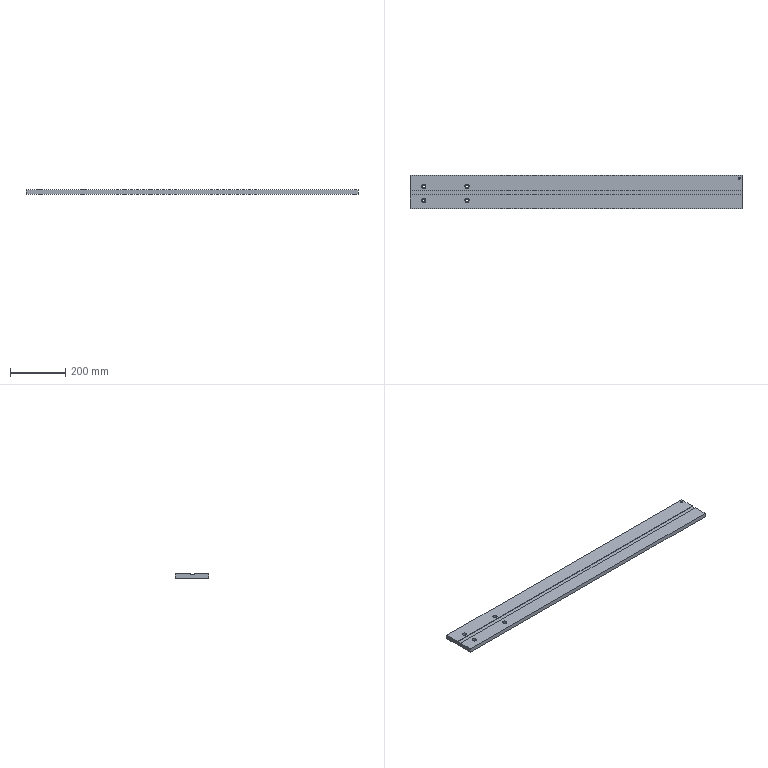Part | SolidWorks | features 3DProfileFeature 2, HoleWzd 2, Extrusion 1, ICE 1 | 1 solid | 35 faces | box 1200 x 120 x 15 mm | volume 2114705 mm3 | cylinder 20 | plane 15 | commonest cylinder face diameters 9 x8 15 x8 6.6 x2 11 x2
STEP:
#1=CARTESIAN_POINT('',(-557.5,20.,-1.5));
#2=VERTEX_POINT('',#1);
#3=CARTESIAN_POINT('',(-542.5,20.,-1.5));
#4=VERTEX_POINT('',#3);
#5=CARTESIAN_POINT('',(-550.,20.,-1.5));
#6=DIRECTION('',(0.,0.,1.));
#7=DIRECTION('',(1.,0.,0.));
#8=AXIS2_PLACEMENT_3D('',#5,#6,#7);
#9=CIRCLE('',#8,7.5);
#10=EDGE_CURVE('',#2,#4,#9,.T.);
#11=ORIENTED_EDGE('',*,*,#10,.F.);
#12=CARTESIAN_POINT('',(-557.5,20.,7.5));
#13=VERTEX_POINT('',#12);
#14=CARTESIAN_POINT('',(-557.5,20.,7.5));
#15=DIRECTION('',(0.,0.,1.));
#16=VECTOR('',#15,1000.);
#17=LINE('',#14,#16);
#18=EDGE_CURVE('',#2,#13,#17,.T.);
#19=ORIENTED_EDGE('',*,*,#18,.T.);
#20=CARTESIAN_POINT('',(-542.5,20.,7.5));
#21=VERTEX_POINT('',#20);
#22=CARTESIAN_POINT('',(-550.,20.,7.5));
#23=DIRECTION('',(0.,0.,1.));
#24=DIRECTION('',(1.,0.,0.));
#25=AXIS2_PLACEMENT_3D('',#22,#23,#24);
#26=CIRCLE('',#25,7.5);
#27=EDGE_CURVE('',#13,#21,#26,.T.);
#28=ORIENTED_EDGE('',*,*,#27,.T.);
#29=CARTESIAN_POINT('',(-542.5,20.,7.5));
#30=DIRECTION('',(0.,0.,1.));
#31=VECTOR('',#30,1000.);
#32=LINE('',#29,#31);
#33=EDGE_CURVE('',#4,#21,#32,.T.);
#34=ORIENTED_EDGE('',*,*,#33,.F.);
#35=EDGE_LOOP('',(#11,#19,#28,#34));
#36=FACE_OUTER_BOUND('',#35,.T.);
#37=CARTESIAN_POINT('',(-550.,20.,7.5));
#38=DIRECTION('',(0.,0.,1.));
#39=DIRECTION('',(1.,0.,0.));
#40=AXIS2_PLACEMENT_3D('',#37,#38,#39);
#41=CYLINDRICAL_SURFACE('',#40,7.5);
#42=ADVANCED_FACE('',(#36),#41,.F.);
#43=CARTESIAN_POINT('',(-554.5,20.,-7.5));
#44=VERTEX_POINT('',#43);
#45=CARTESIAN_POINT('',(-545.5,20.,-7.5));
#46=VERTEX_POINT('',#45);
#47=CARTESIAN_POINT('',(-550.,20.,-7.5));
#48=DIRECTION('',(0.,0.,1.));
#49=DIRECTION('',(1.,0.,0.));
#50=AXIS2_PLACEMENT_3D('',#47,#48,#49);
#51=CIRCLE('',#50,4.5);
#52=EDGE_CURVE('',#44,#46,#51,.T.);
#53=ORIENTED_EDGE('',*,*,#52,.F.);
#54=CARTESIAN_POINT('',(-554.5,20.,-1.5));
#55=VERTEX_POINT('',#54);
#56=CARTESIAN_POINT('',(-554.5,20.,7.5));
#57=DIRECTION('',(0.,0.,1.));
#58=VECTOR('',#57,1000.);
#59=LINE('',#56,#58);
#60=EDGE_CURVE('',#44,#55,#59,.T.);
#61=ORIENTED_EDGE('',*,*,#60,.T.);
#62=CARTESIAN_POINT('',(-545.5,20.,-1.5));
#63=VERTEX_POINT('',#62);
#64=CARTESIAN_POINT('',(-550.,20.,-1.5));
#65=DIRECTION('',(0.,0.,1.));
#66=DIRECTION('',(1.,0.,0.));
#67=AXIS2_PLACEMENT_3D('',#64,#65,#66);
#68=CIRCLE('',#67,4.5);
#69=EDGE_CURVE('',#55,#63,#68,.T.);
#70=ORIENTED_EDGE('',*,*,#69,.T.);
#71=CARTESIAN_POINT('',(-545.5,20.,7.5));
#72=DIRECTION('',(0.,0.,1.));
#73=VECTOR('',#72,1000.);
#74=LINE('',#71,#73);
#75=EDGE_CURVE('',#46,#63,#74,.T.);
#76=ORIENTED_EDGE('',*,*,#75,.F.);
#77=EDGE_LOOP('',(#53,#61,#70,#76));
#78=FACE_OUTER_BOUND('',#77,.T.);
#79=CARTESIAN_POINT('',(-550.,20.,7.5));
#80=DIRECTION('',(0.,0.,1.));
#81=DIRECTION('',(1.,0.,0.));
#82=AXIS2_PLACEMENT_3D('',#79,#80,#81);
#83=CYLINDRICAL_SURFACE('',#82,4.5);
#84=ADVANCED_FACE('',(#78),#83,.F.);
#85=CARTESIAN_POINT('',(-401.5,20.,-1.5));
#86=VERTEX_POINT('',#85);
#87=CARTESIAN_POINT('',(-386.5,20.,-1.5));
#88=VERTEX_POINT('',#87);
#89=CARTESIAN_POINT('',(-394.,20.,-1.5));
#90=DIRECTION('',(0.,0.,1.));
#91=DIRECTION('',(1.,0.,0.));
#92=AXIS2_PLACEMENT_3D('',#89,#90,#91);
#93=CIRCLE('',#92,7.5);
#94=EDGE_CURVE('',#86,#88,#93,.T.);
#95=ORIENTED_EDGE('',*,*,#94,.F.);
#96=CARTESIAN_POINT('',(-401.5,20.,7.5));
#97=VERTEX_POINT('',#96);
#98=CARTESIAN_POINT('',(-401.5,20.,7.5));
#99=DIRECTION('',(0.,0.,1.));
#100=VECTOR('',#99,1000.);
#101=LINE('',#98,#100);
#102=EDGE_CURVE('',#86,#97,#101,.T.);
#103=ORIENTED_EDGE('',*,*,#102,.T.);
#104=CARTESIAN_POINT('',(-386.5,20.,7.5));
#105=VERTEX_POINT('',#104);
#106=CARTESIAN_POINT('',(-394.,20.,7.5));
#107=DIRECTION('',(0.,0.,1.));
#108=DIRECTION('',(1.,0.,0.));
#109=AXIS2_PLACEMENT_3D('',#106,#107,#108);
#110=CIRCLE('',#109,7.5);
#111=EDGE_CURVE('',#97,#105,#110,.T.);
#112=ORIENTED_EDGE('',*,*,#111,.T.);
#113=CARTESIAN_POINT('',(-386.5,20.,7.5));
#114=DIRECTION('',(0.,0.,1.));
#115=VECTOR('',#114,1000.);
#116=LINE('',#113,#115);
#117=EDGE_CURVE('',#88,#105,#116,.T.);
#118=ORIENTED_EDGE('',*,*,#117,.F.);
#119=EDGE_LOOP('',(#95,#103,#112,#118));
#120=FACE_OUTER_BOUND('',#119,.T.);
#121=CARTESIAN_POINT('',(-394.,20.,7.5));
#122=DIRECTION('',(0.,0.,1.));
#123=DIRECTION('',(1.,0.,0.));
#124=AXIS2_PLACEMENT_3D('',#121,#122,#123);
#125=CYLINDRICAL_SURFACE('',#124,7.5);
#126=ADVANCED_FACE('',(#120),#125,.F.);
#127=CARTESIAN_POINT('',(-398.5,20.,-7.5));
#128=VERTEX_POINT('',#127);
#129=CARTESIAN_POINT('',(-389.5,20.,-7.5));
#130=VERTEX_POINT('',#129);
#131=CARTESIAN_POINT('',(-394.,20.,-7.5));
#132=DIRECTION('',(0.,0.,1.));
#133=DIRECTION('',(1.,0.,0.));
#134=AXIS2_PLACEMENT_3D('',#131,#132,#133);
#135=CIRCLE('',#134,4.5);
#136=EDGE_CURVE('',#128,#130,#135,.T.);
#137=ORIENTED_EDGE('',*,*,#136,.F.);
#138=CARTESIAN_POINT('',(-398.5,20.,-1.5));
#139=VERTEX_POINT('',#138);
#140=CARTESIAN_POINT('',(-398.5,20.,7.5));
#141=DIRECTION('',(0.,0.,1.));
#142=VECTOR('',#141,1000.);
#143=LINE('',#140,#142);
#144=EDGE_CURVE('',#128,#139,#143,.T.);
#145=ORIENTED_EDGE('',*,*,#144,.T.);
#146=CARTESIAN_POINT('',(-389.5,20.,-1.5));
#147=VERTEX_POINT('',#146);
#148=CARTESIAN_POINT('',(-394.,20.,-1.5));
#149=DIRECTION('',(0.,0.,1.));
#150=DIRECTION('',(1.,0.,0.));
#151=AXIS2_PLACEMENT_3D('',#148,#149,#150);
#152=CIRCLE('',#151,4.5);
#153=EDGE_CURVE('',#139,#147,#152,.T.);
#154=ORIENTED_EDGE('',*,*,#153,.T.);
#155=CARTESIAN_POINT('',(-389.5,20.,7.5));
#156=DIRECTION('',(0.,0.,1.));
#157=VECTOR('',#156,1000.);
#158=LINE('',#155,#157);
#159=EDGE_CURVE('',#130,#147,#158,.T.);
#160=ORIENTED_EDGE('',*,*,#159,.F.);
#161=EDGE_LOOP('',(#137,#145,#154,#160));
#162=FACE_OUTER_BOUND('',#161,.T.);
#163=CARTESIAN_POINT('',(-394.,20.,7.5));
#164=DIRECTION('',(0.,0.,1.));
#165=DIRECTION('',(1.,0.,0.));
#166=AXIS2_PLACEMENT_3D('',#163,#164,#165);
#167=CYLINDRICAL_SURFACE('',#166,4.5);
#168=ADVANCED_FACE('',(#162),#167,.F.);
#169=CARTESIAN_POINT('',(-401.5,-30.,-1.5));
#170=VERTEX_POINT('',#169);
#171=CARTESIAN_POINT('',(-386.5,-30.,-1.5));
#172=VERTEX_POINT('',#171);
#173=CARTESIAN_POINT('',(-394.,-30.,-1.5));
#174=DIRECTION('',(0.,0.,1.));
#175=DIRECTION('',(1.,0.,0.));
#176=AXIS2_PLACEMENT_3D('',#173,#174,#175);
#177=CIRCLE('',#176,7.5);
#178=EDGE_CURVE('',#170,#172,#177,.T.);
#179=ORIENTED_EDGE('',*,*,#178,.F.);
#180=CARTESIAN_POINT('',(-401.5,-30.,7.5));
#181=VERTEX_POINT('',#180);
#182=CARTESIAN_POINT('',(-401.5,-30.,7.5));
#183=DIRECTION('',(0.,0.,1.));
#184=VECTOR('',#183,1000.);
#185=LINE('',#182,#184);
#186=EDGE_CURVE('',#170,#181,#185,.T.);
#187=ORIENTED_EDGE('',*,*,#186,.T.);
#188=CARTESIAN_POINT('',(-386.5,-30.,7.5));
#189=VERTEX_POINT('',#188);
#190=CARTESIAN_POINT('',(-394.,-30.,7.5));
#191=DIRECTION('',(0.,0.,1.));
#192=DIRECTION('',(1.,0.,0.));
#193=AXIS2_PLACEMENT_3D('',#190,#191,#192);
#194=CIRCLE('',#193,7.5);
#195=EDGE_CURVE('',#181,#189,#194,.T.);
#196=ORIENTED_EDGE('',*,*,#195,.T.);
#197=CARTESIAN_POINT('',(-386.5,-30.,7.5));
#198=DIRECTION('',(0.,0.,1.));
#199=VECTOR('',#198,1000.);
#200=LINE('',#197,#199);
#201=EDGE_CURVE('',#172,#189,#200,.T.);
#202=ORIENTED_EDGE('',*,*,#201,.F.);
#203=EDGE_LOOP('',(#179,#187,#196,#202));
#204=FACE_OUTER_BOUND('',#203,.T.);
#205=CARTESIAN_POINT('',(-394.,-30.,7.5));
#206=DIRECTION('',(0.,0.,1.));
#207=DIRECTION('',(1.,0.,0.));
#208=AXIS2_PLACEMENT_3D('',#205,#206,#207);
#209=CYLINDRICAL_SURFACE('',#208,7.5);
#210=ADVANCED_FACE('',(#204),#209,.F.);
#211=CARTESIAN_POINT('',(-398.5,-30.,-7.5));
#212=VERTEX_POINT('',#211);
#213=CARTESIAN_POINT('',(-389.5,-30.,-7.5));
#214=VERTEX_POINT('',#213);
#215=CARTESIAN_POINT('',(-394.,-30.,-7.5));
#216=DIRECTION('',(0.,0.,1.));
#217=DIRECTION('',(1.,0.,0.));
#218=AXIS2_PLACEMENT_3D('',#215,#216,#217);
#219=CIRCLE('',#218,4.5);
#220=EDGE_CURVE('',#212,#214,#219,.T.);
#221=ORIENTED_EDGE('',*,*,#220,.F.);
#222=CARTESIAN_POINT('',(-398.5,-30.,-1.5));
#223=VERTEX_POINT('',#222);
#224=CARTESIAN_POINT('',(-398.5,-30.,7.5));
#225=DIRECTION('',(0.,0.,1.));
#226=VECTOR('',#225,1000.);
#227=LINE('',#224,#226);
#228=EDGE_CURVE('',#212,#223,#227,.T.);
#229=ORIENTED_EDGE('',*,*,#228,.T.);
#230=CARTESIAN_POINT('',(-389.5,-30.,-1.5));
#231=VERTEX_POINT('',#230);
#232=CARTESIAN_POINT('',(-394.,-30.,-1.5));
#233=DIRECTION('',(0.,0.,1.));
#234=DIRECTION('',(1.,0.,0.));
#235=AXIS2_PLACEMENT_3D('',#232,#233,#234);
#236=CIRCLE('',#235,4.5);
#237=EDGE_CURVE('',#223,#231,#236,.T.);
#238=ORIENTED_EDGE('',*,*,#237,.T.);
#239=CARTESIAN_POINT('',(-389.5,-30.,7.5));
#240=DIRECTION('',(0.,0.,1.));
#241=VECTOR('',#240,1000.);
#242=LINE('',#239,#241);
#243=EDGE_CURVE('',#214,#231,#242,.T.);
#244=ORIENTED_EDGE('',*,*,#243,.F.);
#245=EDGE_LOOP('',(#221,#229,#238,#244));
#246=FACE_OUTER_BOUND('',#245,.T.);
#247=CARTESIAN_POINT('',(-394.,-30.,7.5));
#248=DIRECTION('',(0.,0.,1.));
#249=DIRECTION('',(1.,0.,0.));
#250=AXIS2_PLACEMENT_3D('',#247,#248,#249);
#251=CYLINDRICAL_SURFACE('',#250,4.5);
#252=ADVANCED_FACE('',(#246),#251,.F.);
#253=CARTESIAN_POINT('',(-557.5,-30.,-1.5));
#254=VERTEX_POINT('',#253);
#255=CARTESIAN_POINT('',(-542.5,-30.,-1.5));
#256=VERTEX_POINT('',#255);
#257=CARTESIAN_POINT('',(-550.,-30.,-1.5));
#258=DIRECTION('',(0.,0.,1.));
#259=DIRECTION('',(1.,0.,0.));
#260=AXIS2_PLACEMENT_3D('',#257,#258,#259);
#261=CIRCLE('',#260,7.5);
#262=EDGE_CURVE('',#254,#256,#261,.T.);
#263=ORIENTED_EDGE('',*,*,#262,.F.);
#264=CARTESIAN_POINT('',(-557.5,-30.,7.5));
#265=VERTEX_POINT('',#264);
#266=CARTESIAN_POINT('',(-557.5,-30.,7.5));
#267=DIRECTION('',(0.,0.,1.));
#268=VECTOR('',#267,1000.);
#269=LINE('',#266,#268);
#270=EDGE_CURVE('',#254,#265,#269,.T.);
#271=ORIENTED_EDGE('',*,*,#270,.T.);
#272=CARTESIAN_POINT('',(-542.5,-30.,7.5));
#273=VERTEX_POINT('',#272);
#274=CARTESIAN_POINT('',(-550.,-30.,7.5));
#275=DIRECTION('',(0.,0.,1.));
#276=DIRECTION('',(1.,0.,0.));
#277=AXIS2_PLACEMENT_3D('',#274,#275,#276);
#278=CIRCLE('',#277,7.5);
#279=EDGE_CURVE('',#265,#273,#278,.T.);
#280=ORIENTED_EDGE('',*,*,#279,.T.);
#281=CARTESIAN_POINT('',(-542.5,-30.,7.5));
#282=DIRECTION('',(0.,0.,1.));
#283=VECTOR('',#282,1000.);
#284=LINE('',#281,#283);
#285=EDGE_CURVE('',#256,#273,#284,.T.);
#286=ORIENTED_EDGE('',*,*,#285,.F.);
#287=EDGE_LOOP('',(#263,#271,#280,#286));
#288=FACE_OUTER_BOUND('',#287,.T.);
#289=CARTESIAN_POINT('',(-550.,-30.,7.5));
#290=DIRECTION('',(0.,0.,1.));
#291=DIRECTION('',(1.,0.,0.));
#292=AXIS2_PLACEMENT_3D('',#289,#290,#291);
#293=CYLINDRICAL_SURFACE('',#292,7.5);
#294=ADVANCED_FACE('',(#288),#293,.F.);
#295=CARTESIAN_POINT('',(-554.5,-30.,-7.5));
#296=VERTEX_POINT('',#295);
#297=CARTESIAN_POINT('',(-545.5,-30.,-7.5));
#298=VERTEX_POINT('',#297);
#299=CARTESIAN_POINT('',(-550.,-30.,-7.5));
#300=DIRECTION('',(0.,0.,1.));
#301=DIRECTION('',(1.,0.,0.));
#302=AXIS2_PLACEMENT_3D('',#299,#300,#301);
#303=CIRCLE('',#302,4.5);
#304=EDGE_CURVE('',#296,#298,#303,.T.);
#305=ORIENTED_EDGE('',*,*,#304,.F.);
#306=CARTESIAN_POINT('',(-554.5,-30.,-1.5));
#307=VERTEX_POINT('',#306);
#308=CARTESIAN_POINT('',(-554.5,-30.,7.5));
#309=DIRECTION('',(0.,0.,1.));
#310=VECTOR('',#309,1000.);
#311=LINE('',#308,#310);
#312=EDGE_CURVE('',#296,#307,#311,.T.);
#313=ORIENTED_EDGE('',*,*,#312,.T.);
#314=CARTESIAN_POINT('',(-545.5,-30.,-1.5));
#315=VERTEX_POINT('',#314);
#316=CARTESIAN_POINT('',(-550.,-30.,-1.5));
#317=DIRECTION('',(0.,0.,1.));
#318=DIRECTION('',(1.,0.,0.));
#319=AXIS2_PLACEMENT_3D('',#316,#317,#318);
#320=CIRCLE('',#319,4.5);
#321=EDGE_CURVE('',#307,#315,#320,.T.);
#322=ORIENTED_EDGE('',*,*,#321,.T.);
#323=CARTESIAN_POINT('',(-545.5,-30.,7.5));
#324=DIRECTION('',(0.,0.,1.));
#325=VECTOR('',#324,1000.);
#326=LINE('',#323,#325);
#327=EDGE_CURVE('',#298,#315,#326,.T.);
#328=ORIENTED_EDGE('',*,*,#327,.F.);
#329=EDGE_LOOP('',(#305,#313,#322,#328));
#330=FACE_OUTER_BOUND('',#329,.T.);
#331=CARTESIAN_POINT('',(-550.,-30.,7.5));
#332=DIRECTION('',(0.,0.,1.));
#333=DIRECTION('',(1.,0.,0.));
#334=AXIS2_PLACEMENT_3D('',#331,#332,#333);
#335=CYLINDRICAL_SURFACE('',#334,4.5);
#336=ADVANCED_FACE('',(#330),#335,.F.);
#337=CARTESIAN_POINT('',(595.5,50.,-0.7));
#338=VERTEX_POINT('',#337);
#339=CARTESIAN_POINT('',(584.5,50.,-0.7));
#340=VERTEX_POINT('',#339);
#341=CARTESIAN_POINT('',(590.,50.,-0.7));
#342=DIRECTION('',(0.,0.,-1.));
#343=DIRECTION('',(-1.,0.,0.));
#344=AXIS2_PLACEMENT_3D('',#341,#342,#343);
#345=CIRCLE('',#344,5.5);
#346=EDGE_CURVE('',#338,#340,#345,.T.);
#347=ORIENTED_EDGE('',*,*,#346,.F.);
#348=CARTESIAN_POINT('',(595.5,50.,-7.5));
#349=VERTEX_POINT('',#348);
#350=CARTESIAN_POINT('',(595.5,50.,-7.5));
#351=DIRECTION('',(0.,0.,-1.));
#352=VECTOR('',#351,1000.);
#353=LINE('',#350,#352);
#354=EDGE_CURVE('',#338,#349,#353,.T.);
#355=ORIENTED_EDGE('',*,*,#354,.T.);
#356=CARTESIAN_POINT('',(584.5,50.,-7.5));
#357=VERTEX_POINT('',#356);
#358=CARTESIAN_POINT('',(590.,50.,-7.5));
#359=DIRECTION('',(0.,0.,-1.));
#360=DIRECTION('',(-1.,0.,0.));
#361=AXIS2_PLACEMENT_3D('',#358,#359,#360);
#362=CIRCLE('',#361,5.5);
#363=EDGE_CURVE('',#349,#357,#362,.T.);
#364=ORIENTED_EDGE('',*,*,#363,.T.);
#365=CARTESIAN_POINT('',(584.5,50.,-7.5));
#366=DIRECTION('',(0.,0.,-1.));
#367=VECTOR('',#366,1000.);
#368=LINE('',#365,#367);
#369=EDGE_CURVE('',#340,#357,#368,.T.);
#370=ORIENTED_EDGE('',*,*,#369,.F.);
#371=EDGE_LOOP('',(#347,#355,#364,#370));
#372=FACE_OUTER_BOUND('',#371,.T.);
#373=CARTESIAN_POINT('',(590.,50.,-7.5));
#374=DIRECTION('',(0.,0.,-1.));
#375=DIRECTION('',(-1.,0.,0.));
#376=AXIS2_PLACEMENT_3D('',#373,#374,#375);
#377=CYLINDRICAL_SURFACE('',#376,5.5);
#378=ADVANCED_FACE('',(#372),#377,.F.);
#379=CARTESIAN_POINT('',(593.3,50.,7.5));
#380=VERTEX_POINT('',#379);
#381=CARTESIAN_POINT('',(586.7,50.,7.5));
#382=VERTEX_POINT('',#381);
#383=CARTESIAN_POINT('',(590.,50.,7.5));
#384=DIRECTION('',(0.,0.,-1.));
#385=DIRECTION('',(-1.,0.,0.));
#386=AXIS2_PLACEMENT_3D('',#383,#384,#385);
#387=CIRCLE('',#386,3.3);
#388=EDGE_CURVE('',#380,#382,#387,.T.);
#389=ORIENTED_EDGE('',*,*,#388,.F.);
#390=CARTESIAN_POINT('',(593.3,50.,-0.7));
#391=VERTEX_POINT('',#390);
#392=CARTESIAN_POINT('',(593.3,50.,-7.5));
#393=DIRECTION('',(0.,0.,-1.));
#394=VECTOR('',#393,1000.);
#395=LINE('',#392,#394);
#396=EDGE_CURVE('',#380,#391,#395,.T.);
#397=ORIENTED_EDGE('',*,*,#396,.T.);
#398=CARTESIAN_POINT('',(586.7,50.,-0.7));
#399=VERTEX_POINT('',#398);
#400=CARTESIAN_POINT('',(590.,50.,-0.7));
#401=DIRECTION('',(0.,0.,-1.));
#402=DIRECTION('',(-1.,0.,0.));
#403=AXIS2_PLACEMENT_3D('',#400,#401,#402);
#404=CIRCLE('',#403,3.3);
#405=EDGE_CURVE('',#391,#399,#404,.T.);
#406=ORIENTED_EDGE('',*,*,#405,.T.);
#407=CARTESIAN_POINT('',(586.7,50.,-7.5));
#408=DIRECTION('',(0.,0.,-1.));
#409=VECTOR('',#408,1000.);
#410=LINE('',#407,#409);
#411=EDGE_CURVE('',#382,#399,#410,.T.);
#412=ORIENTED_EDGE('',*,*,#411,.F.);
#413=EDGE_LOOP('',(#389,#397,#406,#412));
#414=FACE_OUTER_BOUND('',#413,.T.);
#415=CARTESIAN_POINT('',(590.,50.,-7.5));
#416=DIRECTION('',(0.,0.,-1.));
#417=DIRECTION('',(-1.,0.,0.));
#418=AXIS2_PLACEMENT_3D('',#415,#416,#417);
#419=CYLINDRICAL_SURFACE('',#418,3.3);
#420=ADVANCED_FACE('',(#414),#419,.F.);
#421=CARTESIAN_POINT('',(-600.,5.2,7.5));
#422=VERTEX_POINT('',#421);
#423=CARTESIAN_POINT('',(600.,5.2,7.5));
#424=VERTEX_POINT('',#423);
#425=CARTESIAN_POINT('',(-600.,5.2,7.5));
#426=DIRECTION('',(1.,0.,0.));
#427=VECTOR('',#426,1000.);
#428=LINE('',#425,#427);
#429=EDGE_CURVE('',#422,#424,#428,.T.);
#430=ORIENTED_EDGE('',*,*,#429,.T.);
#431=CARTESIAN_POINT('',(600.,60.,7.5));
#432=VERTEX_POINT('',#431);
#433=CARTESIAN_POINT('',(600.,60.,7.5));
#434=DIRECTION('',(0.,1.,0.));
#435=VECTOR('',#434,1000.);
#436=LINE('',#433,#435);
#437=EDGE_CURVE('',#424,#432,#436,.T.);
#438=ORIENTED_EDGE('',*,*,#437,.T.);
#439=CARTESIAN_POINT('',(-600.,60.,7.5));
#440=VERTEX_POINT('',#439);
#441=CARTESIAN_POINT('',(-600.,60.,7.5));
#442=DIRECTION('',(-1.,0.,0.));
#443=VECTOR('',#442,1000.);
#444=LINE('',#441,#443);
#445=EDGE_CURVE('',#432,#440,#444,.T.);
#446=ORIENTED_EDGE('',*,*,#445,.T.);
#447=CARTESIAN_POINT('',(-600.,60.,7.5));
#448=DIRECTION('',(0.,-1.,0.));
#449=VECTOR('',#448,1000.);
#450=LINE('',#447,#449);
#451=EDGE_CURVE('',#440,#422,#450,.T.);
#452=ORIENTED_EDGE('',*,*,#451,.T.);
#453=EDGE_LOOP('',(#430,#438,#446,#452));
#454=FACE_OUTER_BOUND('',#453,.T.);
#455=CARTESIAN_POINT('',(590.,50.,7.5));
#456=DIRECTION('',(0.,0.,-1.));
#457=DIRECTION('',(-1.,0.,0.));
#458=AXIS2_PLACEMENT_3D('',#455,#456,#457);
#459=CIRCLE('',#458,3.3);
#460=EDGE_CURVE('',#382,#380,#459,.T.);
#461=ORIENTED_EDGE('',*,*,#460,.T.);
#462=ORIENTED_EDGE('',*,*,#388,.T.);
#463=EDGE_LOOP('',(#461,#462));
#464=FACE_BOUND('',#463,.T.);
#465=CARTESIAN_POINT('',(-394.,20.,7.5));
#466=DIRECTION('',(0.,0.,1.));
#467=DIRECTION('',(1.,0.,0.));
#468=AXIS2_PLACEMENT_3D('',#465,#466,#467);
#469=CIRCLE('',#468,7.5);
#470=EDGE_CURVE('',#105,#97,#469,.T.);
#471=ORIENTED_EDGE('',*,*,#470,.F.);
#472=ORIENTED_EDGE('',*,*,#111,.F.);
#473=EDGE_LOOP('',(#471,#472));
#474=FACE_BOUND('',#473,.T.);
#475=CARTESIAN_POINT('',(-550.,20.,7.5));
#476=DIRECTION('',(0.,0.,1.));
#477=DIRECTION('',(1.,0.,0.));
#478=AXIS2_PLACEMENT_3D('',#475,#476,#477);
#479=CIRCLE('',#478,7.5);
#480=EDGE_CURVE('',#21,#13,#479,.T.);
#481=ORIENTED_EDGE('',*,*,#480,.F.);
#482=ORIENTED_EDGE('',*,*,#27,.F.);
#483=EDGE_LOOP('',(#481,#482));
#484=FACE_BOUND('',#483,.T.);
#485=CARTESIAN_POINT('',(0.,0.,7.5));
#486=DIRECTION('',(0.,0.,1.));
#487=DIRECTION('',(1.,0.,0.));
#488=AXIS2_PLACEMENT_3D('',#485,#486,#487);
#489=PLANE('',#488);
#490=ADVANCED_FACE('',(#454,#464,#474,#484),#489,.T.);
#491=ORIENTED_EDGE('',*,*,#437,.F.);
#492=CARTESIAN_POINT('',(600.,5.2,5.5));
#493=VERTEX_POINT('',#492);
#494=CARTESIAN_POINT('',(600.,5.2,7.5));
#495=DIRECTION('',(0.,0.,1.));
#496=VECTOR('',#495,1000.);
#497=LINE('',#494,#496);
#498=EDGE_CURVE('',#493,#424,#497,.T.);
#499=ORIENTED_EDGE('',*,*,#498,.F.);
#500=CARTESIAN_POINT('',(600.,-10.,5.5));
#501=VERTEX_POINT('',#500);
#502=CARTESIAN_POINT('',(600.,5.2,5.5));
#503=DIRECTION('',(0.,1.,0.));
#504=VECTOR('',#503,1000.);
#505=LINE('',#502,#504);
#506=EDGE_CURVE('',#501,#493,#505,.T.);
#507=ORIENTED_EDGE('',*,*,#506,.F.);
#508=CARTESIAN_POINT('',(600.,-10.,7.5));
#509=VERTEX_POINT('',#508);
#510=CARTESIAN_POINT('',(600.,-10.,7.5));
#511=DIRECTION('',(0.,0.,-1.));
#512=VECTOR('',#511,1000.);
#513=LINE('',#510,#512);
#514=EDGE_CURVE('',#509,#501,#513,.T.);
#515=ORIENTED_EDGE('',*,*,#514,.F.);
#516=CARTESIAN_POINT('',(600.,-60.,7.5));
#517=VERTEX_POINT('',#516);
#518=CARTESIAN_POINT('',(600.,60.,7.5));
#519=DIRECTION('',(0.,1.,0.));
#520=VECTOR('',#519,1000.);
#521=LINE('',#518,#520);
#522=EDGE_CURVE('',#517,#509,#521,.T.);
#523=ORIENTED_EDGE('',*,*,#522,.F.);
#524=CARTESIAN_POINT('',(600.,-60.,-7.5));
#525=VERTEX_POINT('',#524);
#526=CARTESIAN_POINT('',(600.,-60.,7.5));
#527=DIRECTION('',(0.,0.,-1.));
#528=VECTOR('',#527,1000.);
#529=LINE('',#526,#528);
#530=EDGE_CURVE('',#517,#525,#529,.T.);
#531=ORIENTED_EDGE('',*,*,#530,.T.);
#532=CARTESIAN_POINT('',(600.,60.,-7.5));
#533=VERTEX_POINT('',#532);
#534=CARTESIAN_POINT('',(600.,60.,-7.5));
#535=DIRECTION('',(0.,1.,0.));
#536=VECTOR('',#535,1000.);
#537=LINE('',#534,#536);
#538=EDGE_CURVE('',#525,#533,#537,.T.);
#539=ORIENTED_EDGE('',*,*,#538,.T.);
#540=CARTESIAN_POINT('',(600.,60.,7.5));
#541=DIRECTION('',(0.,0.,-1.));
#542=VECTOR('',#541,1000.);
#543=LINE('',#540,#542);
#544=EDGE_CURVE('',#432,#533,#543,.T.);
#545=ORIENTED_EDGE('',*,*,#544,.F.);
#546=EDGE_LOOP('',(#491,#499,#507,#515,#523,#531,#539,#545));
#547=FACE_OUTER_BOUND('',#546,.T.);
#548=CARTESIAN_POINT('',(600.,60.,7.5));
#549=DIRECTION('',(-1.,0.,0.));
#550=DIRECTION('',(0.,0.,1.));
#551=AXIS2_PLACEMENT_3D('',#548,#549,#550);
#552=PLANE('',#551);
#553=ADVANCED_FACE('',(#547),#552,.F.);
#554=CARTESIAN_POINT('',(-600.,60.,-7.5));
#555=VERTEX_POINT('',#554);
#556=CARTESIAN_POINT('',(-600.,60.,-7.5));
#557=DIRECTION('',(-1.,0.,0.));
#558=VECTOR('',#557,1000.);
#559=LINE('',#556,#558);
#560=EDGE_CURVE('',#533,#555,#559,.T.);
#561=ORIENTED_EDGE('',*,*,#560,.T.);
#562=CARTESIAN_POINT('',(-600.,60.,7.5));
#563=DIRECTION('',(0.,0.,-1.));
#564=VECTOR('',#563,1000.);
#565=LINE('',#562,#564);
#566=EDGE_CURVE('',#440,#555,#565,.T.);
#567=ORIENTED_EDGE('',*,*,#566,.F.);
#568=ORIENTED_EDGE('',*,*,#445,.F.);
#569=ORIENTED_EDGE('',*,*,#544,.T.);
#570=EDGE_LOOP('',(#561,#567,#568,#569));
#571=FACE_OUTER_BOUND('',#570,.T.);
#572=CARTESIAN_POINT('',(-600.,60.,7.5));
#573=DIRECTION('',(0.,-1.,0.));
#574=DIRECTION('',(0.,0.,-1.));
#575=AXIS2_PLACEMENT_3D('',#572,#573,#574);
#576=PLANE('',#575);
#577=ADVANCED_FACE('',(#571),#576,.F.);
#578=CARTESIAN_POINT('',(-600.,-10.,5.5));
#579=VERTEX_POINT('',#578);
#580=CARTESIAN_POINT('',(-600.,5.2,5.5));
#581=VERTEX_POINT('',#580);
#582=CARTESIAN_POINT('',(-600.,5.2,5.5));
#583=DIRECTION('',(0.,1.,0.));
#584=VECTOR('',#583,1000.);
#585=LINE('',#582,#584);
#586=EDGE_CURVE('',#579,#581,#585,.T.);
#587=ORIENTED_EDGE('',*,*,#586,.T.);
#588=CARTESIAN_POINT('',(-600.,5.2,7.5));
#589=DIRECTION('',(0.,0.,1.));
#590=VECTOR('',#589,1000.);
#591=LINE('',#588,#590);
#592=EDGE_CURVE('',#581,#422,#591,.T.);
#593=ORIENTED_EDGE('',*,*,#592,.T.);
#594=ORIENTED_EDGE('',*,*,#451,.F.);
#595=ORIENTED_EDGE('',*,*,#566,.T.);
#596=CARTESIAN_POINT('',(-600.,-60.,-7.5));
#597=VERTEX_POINT('',#596);
#598=CARTESIAN_POINT('',(-600.,60.,-7.5));
#599=DIRECTION('',(0.,-1.,0.));
#600=VECTOR('',#599,1000.);
#601=LINE('',#598,#600);
#602=EDGE_CURVE('',#555,#597,#601,.T.);
#603=ORIENTED_EDGE('',*,*,#602,.T.);
#604=CARTESIAN_POINT('',(-600.,-60.,7.5));
#605=VERTEX_POINT('',#604);
#606=CARTESIAN_POINT('',(-600.,-60.,7.5));
#607=DIRECTION('',(0.,0.,-1.));
#608=VECTOR('',#607,1000.);
#609=LINE('',#606,#608);
#610=EDGE_CURVE('',#605,#597,#609,.T.);
#611=ORIENTED_EDGE('',*,*,#610,.F.);
#612=CARTESIAN_POINT('',(-600.,-10.,7.5));
#613=VERTEX_POINT('',#612);
#614=CARTESIAN_POINT('',(-600.,60.,7.5));
#615=DIRECTION('',(0.,-1.,0.));
#616=VECTOR('',#615,1000.);
#617=LINE('',#614,#616);
#618=EDGE_CURVE('',#613,#605,#617,.T.);
#619=ORIENTED_EDGE('',*,*,#618,.F.);
#620=CARTESIAN_POINT('',(-600.,-10.,7.5));
#621=DIRECTION('',(0.,0.,-1.));
#622=VECTOR('',#621,1000.);
#623=LINE('',#620,#622);
#624=EDGE_CURVE('',#613,#579,#623,.T.);
#625=ORIENTED_EDGE('',*,*,#624,.T.);
#626=EDGE_LOOP('',(#587,#593,#594,#595,#603,#611,#619,#625));
#627=FACE_OUTER_BOUND('',#626,.T.);
#628=CARTESIAN_POINT('',(-600.,60.,7.5));
#629=DIRECTION('',(1.,0.,0.));
#630=DIRECTION('',(0.,0.,-1.));
#631=AXIS2_PLACEMENT_3D('',#628,#629,#630);
#632=PLANE('',#631);
#633=ADVANCED_FACE('',(#627),#632,.F.);
#634=CARTESIAN_POINT('',(-600.,-60.,-7.5));
#635=DIRECTION('',(1.,0.,0.));
#636=VECTOR('',#635,1000.);
#637=LINE('',#634,#636);
#638=EDGE_CURVE('',#597,#525,#637,.T.);
#639=ORIENTED_EDGE('',*,*,#638,.T.);
#640=ORIENTED_EDGE('',*,*,#530,.F.);
#641=CARTESIAN_POINT('',(-600.,-60.,7.5));
#642=DIRECTION('',(1.,0.,0.));
#643=VECTOR('',#642,1000.);
#644=LINE('',#641,#643);
#645=EDGE_CURVE('',#605,#517,#644,.T.);
#646=ORIENTED_EDGE('',*,*,#645,.F.);
#647=ORIENTED_EDGE('',*,*,#610,.T.);
#648=EDGE_LOOP('',(#639,#640,#646,#647));
#649=FACE_OUTER_BOUND('',#648,.T.);
#650=CARTESIAN_POINT('',(-600.,-60.,7.5));
#651=DIRECTION('',(0.,1.,0.));
#652=DIRECTION('',(0.,0.,1.));
#653=AXIS2_PLACEMENT_3D('',#650,#651,#652);
#654=PLANE('',#653);
#655=ADVANCED_FACE('',(#649),#654,.F.);
#656=CARTESIAN_POINT('',(-600.,-10.,7.5));
#657=DIRECTION('',(1.,0.,0.));
#658=VECTOR('',#657,1000.);
#659=LINE('',#656,#658);
#660=EDGE_CURVE('',#613,#509,#659,.T.);
#661=ORIENTED_EDGE('',*,*,#660,.F.);
#662=ORIENTED_EDGE('',*,*,#618,.T.);
#663=ORIENTED_EDGE('',*,*,#645,.T.);
#664=ORIENTED_EDGE('',*,*,#522,.T.);
#665=EDGE_LOOP('',(#661,#662,#663,#664));
#666=FACE_OUTER_BOUND('',#665,.T.);
#667=CARTESIAN_POINT('',(-394.,-30.,7.5));
#668=DIRECTION('',(0.,0.,1.));
#669=DIRECTION('',(1.,0.,0.));
#670=AXIS2_PLACEMENT_3D('',#667,#668,#669);
#671=CIRCLE('',#670,7.5);
#672=EDGE_CURVE('',#189,#181,#671,.T.);
#673=ORIENTED_EDGE('',*,*,#672,.F.);
#674=ORIENTED_EDGE('',*,*,#195,.F.);
#675=EDGE_LOOP('',(#673,#674));
#676=FACE_BOUND('',#675,.T.);
#677=CARTESIAN_POINT('',(-550.,-30.,7.5));
#678=DIRECTION('',(0.,0.,1.));
#679=DIRECTION('',(1.,0.,0.));
#680=AXIS2_PLACEMENT_3D('',#677,#678,#679);
#681=CIRCLE('',#680,7.5);
#682=EDGE_CURVE('',#273,#265,#681,.T.);
#683=ORIENTED_EDGE('',*,*,#682,.F.);
#684=ORIENTED_EDGE('',*,*,#279,.F.);
#685=EDGE_LOOP('',(#683,#684));
#686=FACE_BOUND('',#685,.T.);
#687=CARTESIAN_POINT('',(0.,0.,7.5));
#688=DIRECTION('',(0.,0.,1.));
#689=DIRECTION('',(1.,0.,0.));
#690=AXIS2_PLACEMENT_3D('',#687,#688,#689);
#691=PLANE('',#690);
#692=ADVANCED_FACE('',(#666,#676,#686),#691,.T.);
#693=CARTESIAN_POINT('',(-550.,20.,-7.5));
#694=DIRECTION('',(0.,0.,1.));
#695=DIRECTION('',(1.,0.,0.));
#696=AXIS2_PLACEMENT_3D('',#693,#694,#695);
#697=CIRCLE('',#696,4.5);
#698=EDGE_CURVE('',#46,#44,#697,.T.);
#699=ORIENTED_EDGE('',*,*,#698,.T.);
#700=ORIENTED_EDGE('',*,*,#52,.T.);
#701=EDGE_LOOP('',(#699,#700));
#702=FACE_BOUND('',#701,.T.);
#703=CARTESIAN_POINT('',(-394.,20.,-7.5));
#704=DIRECTION('',(0.,0.,1.));
#705=DIRECTION('',(1.,0.,0.));
#706=AXIS2_PLACEMENT_3D('',#703,#704,#705);
#707=CIRCLE('',#706,4.5);
#708=EDGE_CURVE('',#130,#128,#707,.T.);
#709=ORIENTED_EDGE('',*,*,#708,.T.);
#710=ORIENTED_EDGE('',*,*,#136,.T.);
#711=EDGE_LOOP('',(#709,#710));
#712=FACE_BOUND('',#711,.T.);
#713=CARTESIAN_POINT('',(-394.,-30.,-7.5));
#714=DIRECTION('',(0.,0.,1.));
#715=DIRECTION('',(1.,0.,0.));
#716=AXIS2_PLACEMENT_3D('',#713,#714,#715);
#717=CIRCLE('',#716,4.5);
#718=EDGE_CURVE('',#214,#212,#717,.T.);
#719=ORIENTED_EDGE('',*,*,#718,.T.);
#720=ORIENTED_EDGE('',*,*,#220,.T.);
#721=EDGE_LOOP('',(#719,#720));
#722=FACE_BOUND('',#721,.T.);
#723=CARTESIAN_POINT('',(-550.,-30.,-7.5));
#724=DIRECTION('',(0.,0.,1.));
#725=DIRECTION('',(1.,0.,0.));
#726=AXIS2_PLACEMENT_3D('',#723,#724,#725);
#727=CIRCLE('',#726,4.5);
#728=EDGE_CURVE('',#298,#296,#727,.T.);
#729=ORIENTED_EDGE('',*,*,#728,.T.);
#730=ORIENTED_EDGE('',*,*,#304,.T.);
#731=EDGE_LOOP('',(#729,#730));
#732=FACE_BOUND('',#731,.T.);
#733=CARTESIAN_POINT('',(590.,50.,-7.5));
#734=DIRECTION('',(0.,0.,-1.));
#735=DIRECTION('',(-1.,0.,0.));
#736=AXIS2_PLACEMENT_3D('',#733,#734,#735);
#737=CIRCLE('',#736,5.5);
#738=EDGE_CURVE('',#357,#349,#737,.T.);
#739=ORIENTED_EDGE('',*,*,#738,.F.);
#740=ORIENTED_EDGE('',*,*,#363,.F.);
#741=EDGE_LOOP('',(#739,#740));
#742=FACE_BOUND('',#741,.T.);
#743=ORIENTED_EDGE('',*,*,#538,.F.);
#744=ORIENTED_EDGE('',*,*,#638,.F.);
#745=ORIENTED_EDGE('',*,*,#602,.F.);
#746=ORIENTED_EDGE('',*,*,#560,.F.);
#747=EDGE_LOOP('',(#743,#744,#745,#746));
#748=FACE_OUTER_BOUND('',#747,.T.);
#749=CARTESIAN_POINT('',(0.,0.,-7.5));
#750=DIRECTION('',(0.,0.,1.));
#751=DIRECTION('',(1.,0.,0.));
#752=AXIS2_PLACEMENT_3D('',#749,#750,#751);
#753=PLANE('',#752);
#754=ADVANCED_FACE('',(#702,#712,#722,#732,#742,#748),#753,.F.);
#755=ORIENTED_EDGE('',*,*,#396,.F.);
#756=ORIENTED_EDGE('',*,*,#460,.F.);
#757=ORIENTED_EDGE('',*,*,#411,.T.);
#758=CARTESIAN_POINT('',(590.,50.,-0.7));
#759=DIRECTION('',(0.,0.,-1.));
#760=DIRECTION('',(-1.,0.,0.));
#761=AXIS2_PLACEMENT_3D('',#758,#759,#760);
#762=CIRCLE('',#761,3.3);
#763=EDGE_CURVE('',#399,#391,#762,.T.);
#764=ORIENTED_EDGE('',*,*,#763,.T.);
#765=EDGE_LOOP('',(#755,#756,#757,#764));
#766=FACE_OUTER_BOUND('',#765,.T.);
#767=CARTESIAN_POINT('',(590.,50.,-7.5));
#768=DIRECTION('',(0.,0.,-1.));
#769=DIRECTION('',(-1.,0.,0.));
#770=AXIS2_PLACEMENT_3D('',#767,#768,#769);
#771=CYLINDRICAL_SURFACE('',#770,3.3);
#772=ADVANCED_FACE('',(#766),#771,.F.);
#773=ORIENTED_EDGE('',*,*,#763,.F.);
#774=ORIENTED_EDGE('',*,*,#405,.F.);
#775=EDGE_LOOP('',(#773,#774));
#776=FACE_BOUND('',#775,.T.);
#777=CARTESIAN_POINT('',(590.,50.,-0.7));
#778=DIRECTION('',(0.,0.,-1.));
#779=DIRECTION('',(-1.,0.,0.));
#780=AXIS2_PLACEMENT_3D('',#777,#778,#779);
#781=CIRCLE('',#780,5.5);
#782=EDGE_CURVE('',#340,#338,#781,.T.);
#783=ORIENTED_EDGE('',*,*,#782,.T.);
#784=ORIENTED_EDGE('',*,*,#346,.T.);
#785=EDGE_LOOP('',(#783,#784));
#786=FACE_OUTER_BOUND('',#785,.T.);
#787=CARTESIAN_POINT('',(593.3,50.,-0.7));
#788=DIRECTION('',(0.,0.,1.));
#789=DIRECTION('',(1.,0.,0.));
#790=AXIS2_PLACEMENT_3D('',#787,#788,#789);
#791=PLANE('',#790);
#792=ADVANCED_FACE('',(#776,#786),#791,.F.);
#793=ORIENTED_EDGE('',*,*,#354,.F.);
#794=ORIENTED_EDGE('',*,*,#782,.F.);
#795=ORIENTED_EDGE('',*,*,#369,.T.);
#796=ORIENTED_EDGE('',*,*,#738,.T.);
#797=EDGE_LOOP('',(#793,#794,#795,#796));
#798=FACE_OUTER_BOUND('',#797,.T.);
#799=CARTESIAN_POINT('',(590.,50.,-7.5));
#800=DIRECTION('',(0.,0.,-1.));
#801=DIRECTION('',(-1.,0.,0.));
#802=AXIS2_PLACEMENT_3D('',#799,#800,#801);
#803=CYLINDRICAL_SURFACE('',#802,5.5);
#804=ADVANCED_FACE('',(#798),#803,.F.);
#805=ORIENTED_EDGE('',*,*,#312,.F.);
#806=ORIENTED_EDGE('',*,*,#728,.F.);
#807=ORIENTED_EDGE('',*,*,#327,.T.);
#808=CARTESIAN_POINT('',(-550.,-30.,-1.5));
#809=DIRECTION('',(0.,0.,1.));
#810=DIRECTION('',(1.,0.,0.));
#811=AXIS2_PLACEMENT_3D('',#808,#809,#810);
#812=CIRCLE('',#811,4.5);
#813=EDGE_CURVE('',#315,#307,#812,.T.);
#814=ORIENTED_EDGE('',*,*,#813,.T.);
#815=EDGE_LOOP('',(#805,#806,#807,#814));
#816=FACE_OUTER_BOUND('',#815,.T.);
#817=CARTESIAN_POINT('',(-550.,-30.,7.5));
#818=DIRECTION('',(0.,0.,1.));
#819=DIRECTION('',(1.,0.,0.));
#820=AXIS2_PLACEMENT_3D('',#817,#818,#819);
#821=CYLINDRICAL_SURFACE('',#820,4.5);
#822=ADVANCED_FACE('',(#816),#821,.F.);
#823=ORIENTED_EDGE('',*,*,#813,.F.);
#824=ORIENTED_EDGE('',*,*,#321,.F.);
#825=EDGE_LOOP('',(#823,#824));
#826=FACE_BOUND('',#825,.T.);
#827=CARTESIAN_POINT('',(-550.,-30.,-1.5));
#828=DIRECTION('',(0.,0.,1.));
#829=DIRECTION('',(1.,0.,0.));
#830=AXIS2_PLACEMENT_3D('',#827,#828,#829);
#831=CIRCLE('',#830,7.5);
#832=EDGE_CURVE('',#256,#254,#831,.T.);
#833=ORIENTED_EDGE('',*,*,#832,.T.);
#834=ORIENTED_EDGE('',*,*,#262,.T.);
#835=EDGE_LOOP('',(#833,#834));
#836=FACE_OUTER_BOUND('',#835,.T.);
#837=CARTESIAN_POINT('',(-545.5,-30.,-1.5));
#838=DIRECTION('',(0.,0.,-1.));
#839=DIRECTION('',(-1.,0.,0.));
#840=AXIS2_PLACEMENT_3D('',#837,#838,#839);
#841=PLANE('',#840);
#842=ADVANCED_FACE('',(#826,#836),#841,.F.);
#843=ORIENTED_EDGE('',*,*,#270,.F.);
#844=ORIENTED_EDGE('',*,*,#832,.F.);
#845=ORIENTED_EDGE('',*,*,#285,.T.);
#846=ORIENTED_EDGE('',*,*,#682,.T.);
#847=EDGE_LOOP('',(#843,#844,#845,#846));
#848=FACE_OUTER_BOUND('',#847,.T.);
#849=CARTESIAN_POINT('',(-550.,-30.,7.5));
#850=DIRECTION('',(0.,0.,1.));
#851=DIRECTION('',(1.,0.,0.));
#852=AXIS2_PLACEMENT_3D('',#849,#850,#851);
#853=CYLINDRICAL_SURFACE('',#852,7.5);
#854=ADVANCED_FACE('',(#848),#853,.F.);
#855=ORIENTED_EDGE('',*,*,#228,.F.);
#856=ORIENTED_EDGE('',*,*,#718,.F.);
#857=ORIENTED_EDGE('',*,*,#243,.T.);
#858=CARTESIAN_POINT('',(-394.,-30.,-1.5));
#859=DIRECTION('',(0.,0.,1.));
#860=DIRECTION('',(1.,0.,0.));
#861=AXIS2_PLACEMENT_3D('',#858,#859,#860);
#862=CIRCLE('',#861,4.5);
#863=EDGE_CURVE('',#231,#223,#862,.T.);
#864=ORIENTED_EDGE('',*,*,#863,.T.);
#865=EDGE_LOOP('',(#855,#856,#857,#864));
#866=FACE_OUTER_BOUND('',#865,.T.);
#867=CARTESIAN_POINT('',(-394.,-30.,7.5));
#868=DIRECTION('',(0.,0.,1.));
#869=DIRECTION('',(1.,0.,0.));
#870=AXIS2_PLACEMENT_3D('',#867,#868,#869);
#871=CYLINDRICAL_SURFACE('',#870,4.5);
#872=ADVANCED_FACE('',(#866),#871,.F.);
#873=ORIENTED_EDGE('',*,*,#863,.F.);
#874=ORIENTED_EDGE('',*,*,#237,.F.);
#875=EDGE_LOOP('',(#873,#874));
#876=FACE_BOUND('',#875,.T.);
#877=CARTESIAN_POINT('',(-394.,-30.,-1.5));
#878=DIRECTION('',(0.,0.,1.));
#879=DIRECTION('',(1.,0.,0.));
#880=AXIS2_PLACEMENT_3D('',#877,#878,#879);
#881=CIRCLE('',#880,7.5);
#882=EDGE_CURVE('',#172,#170,#881,.T.);
#883=ORIENTED_EDGE('',*,*,#882,.T.);
#884=ORIENTED_EDGE('',*,*,#178,.T.);
#885=EDGE_LOOP('',(#883,#884));
#886=FACE_OUTER_BOUND('',#885,.T.);
#887=CARTESIAN_POINT('',(-389.5,-30.,-1.5));
#888=DIRECTION('',(0.,0.,-1.));
#889=DIRECTION('',(-1.,0.,0.));
#890=AXIS2_PLACEMENT_3D('',#887,#888,#889);
#891=PLANE('',#890);
#892=ADVANCED_FACE('',(#876,#886),#891,.F.);
#893=ORIENTED_EDGE('',*,*,#186,.F.);
#894=ORIENTED_EDGE('',*,*,#882,.F.);
#895=ORIENTED_EDGE('',*,*,#201,.T.);
#896=ORIENTED_EDGE('',*,*,#672,.T.);
#897=EDGE_LOOP('',(#893,#894,#895,#896));
#898=FACE_OUTER_BOUND('',#897,.T.);
#899=CARTESIAN_POINT('',(-394.,-30.,7.5));
#900=DIRECTION('',(0.,0.,1.));
#901=DIRECTION('',(1.,0.,0.));
#902=AXIS2_PLACEMENT_3D('',#899,#900,#901);
#903=CYLINDRICAL_SURFACE('',#902,7.5);
#904=ADVANCED_FACE('',(#898),#903,.F.);
#905=ORIENTED_EDGE('',*,*,#144,.F.);
#906=ORIENTED_EDGE('',*,*,#708,.F.);
#907=ORIENTED_EDGE('',*,*,#159,.T.);
#908=CARTESIAN_POINT('',(-394.,20.,-1.5));
#909=DIRECTION('',(0.,0.,1.));
#910=DIRECTION('',(1.,0.,0.));
#911=AXIS2_PLACEMENT_3D('',#908,#909,#910);
#912=CIRCLE('',#911,4.5);
#913=EDGE_CURVE('',#147,#139,#912,.T.);
#914=ORIENTED_EDGE('',*,*,#913,.T.);
#915=EDGE_LOOP('',(#905,#906,#907,#914));
#916=FACE_OUTER_BOUND('',#915,.T.);
#917=CARTESIAN_POINT('',(-394.,20.,7.5));
#918=DIRECTION('',(0.,0.,1.));
#919=DIRECTION('',(1.,0.,0.));
#920=AXIS2_PLACEMENT_3D('',#917,#918,#919);
#921=CYLINDRICAL_SURFACE('',#920,4.5);
#922=ADVANCED_FACE('',(#916),#921,.F.);
#923=ORIENTED_EDGE('',*,*,#913,.F.);
#924=ORIENTED_EDGE('',*,*,#153,.F.);
#925=EDGE_LOOP('',(#923,#924));
#926=FACE_BOUND('',#925,.T.);
#927=CARTESIAN_POINT('',(-394.,20.,-1.5));
#928=DIRECTION('',(0.,0.,1.));
#929=DIRECTION('',(1.,0.,0.));
#930=AXIS2_PLACEMENT_3D('',#927,#928,#929);
#931=CIRCLE('',#930,7.5);
#932=EDGE_CURVE('',#88,#86,#931,.T.);
#933=ORIENTED_EDGE('',*,*,#932,.T.);
#934=ORIENTED_EDGE('',*,*,#94,.T.);
#935=EDGE_LOOP('',(#933,#934));
#936=FACE_OUTER_BOUND('',#935,.T.);
#937=CARTESIAN_POINT('',(-389.5,20.,-1.5));
#938=DIRECTION('',(0.,0.,-1.));
#939=DIRECTION('',(-1.,0.,0.));
#940=AXIS2_PLACEMENT_3D('',#937,#938,#939);
#941=PLANE('',#940);
#942=ADVANCED_FACE('',(#926,#936),#941,.F.);
#943=ORIENTED_EDGE('',*,*,#102,.F.);
#944=ORIENTED_EDGE('',*,*,#932,.F.);
#945=ORIENTED_EDGE('',*,*,#117,.T.);
#946=ORIENTED_EDGE('',*,*,#470,.T.);
#947=EDGE_LOOP('',(#943,#944,#945,#946));
#948=FACE_OUTER_BOUND('',#947,.T.);
#949=CARTESIAN_POINT('',(-394.,20.,7.5));
#950=DIRECTION('',(0.,0.,1.));
#951=DIRECTION('',(1.,0.,0.));
#952=AXIS2_PLACEMENT_3D('',#949,#950,#951);
#953=CYLINDRICAL_SURFACE('',#952,7.5);
#954=ADVANCED_FACE('',(#948),#953,.F.);
#955=ORIENTED_EDGE('',*,*,#60,.F.);
#956=ORIENTED_EDGE('',*,*,#698,.F.);
#957=ORIENTED_EDGE('',*,*,#75,.T.);
#958=CARTESIAN_POINT('',(-550.,20.,-1.5));
#959=DIRECTION('',(0.,0.,1.));
#960=DIRECTION('',(1.,0.,0.));
#961=AXIS2_PLACEMENT_3D('',#958,#959,#960);
#962=CIRCLE('',#961,4.5);
#963=EDGE_CURVE('',#63,#55,#962,.T.);
#964=ORIENTED_EDGE('',*,*,#963,.T.);
#965=EDGE_LOOP('',(#955,#956,#957,#964));
#966=FACE_OUTER_BOUND('',#965,.T.);
#967=CARTESIAN_POINT('',(-550.,20.,7.5));
#968=DIRECTION('',(0.,0.,1.));
#969=DIRECTION('',(1.,0.,0.));
#970=AXIS2_PLACEMENT_3D('',#967,#968,#969);
#971=CYLINDRICAL_SURFACE('',#970,4.5);
#972=ADVANCED_FACE('',(#966),#971,.F.);
#973=ORIENTED_EDGE('',*,*,#963,.F.);
#974=ORIENTED_EDGE('',*,*,#69,.F.);
#975=EDGE_LOOP('',(#973,#974));
#976=FACE_BOUND('',#975,.T.);
#977=CARTESIAN_POINT('',(-550.,20.,-1.5));
#978=DIRECTION('',(0.,0.,1.));
#979=DIRECTION('',(1.,0.,0.));
#980=AXIS2_PLACEMENT_3D('',#977,#978,#979);
#981=CIRCLE('',#980,7.5);
#982=EDGE_CURVE('',#4,#2,#981,.T.);
#983=ORIENTED_EDGE('',*,*,#982,.T.);
#984=ORIENTED_EDGE('',*,*,#10,.T.);
#985=EDGE_LOOP('',(#983,#984));
#986=FACE_OUTER_BOUND('',#985,.T.);
#987=CARTESIAN_POINT('',(-545.5,20.,-1.5));
#988=DIRECTION('',(0.,0.,-1.));
#989=DIRECTION('',(-1.,0.,0.));
#990=AXIS2_PLACEMENT_3D('',#987,#988,#989);
#991=PLANE('',#990);
#992=ADVANCED_FACE('',(#976,#986),#991,.F.);
#993=ORIENTED_EDGE('',*,*,#18,.F.);
#994=ORIENTED_EDGE('',*,*,#982,.F.);
#995=ORIENTED_EDGE('',*,*,#33,.T.);
#996=ORIENTED_EDGE('',*,*,#480,.T.);
#997=EDGE_LOOP('',(#993,#994,#995,#996));
#998=FACE_OUTER_BOUND('',#997,.T.);
#999=CARTESIAN_POINT('',(-550.,20.,7.5));
#1000=DIRECTION('',(0.,0.,1.));
#1001=DIRECTION('',(1.,0.,0.));
#1002=AXIS2_PLACEMENT_3D('',#999,#1000,#1001);
#1003=CYLINDRICAL_SURFACE('',#1002,7.5);
#1004=ADVANCED_FACE('',(#998),#1003,.F.);
#1005=ORIENTED_EDGE('',*,*,#498,.T.);
#1006=ORIENTED_EDGE('',*,*,#429,.F.);
#1007=ORIENTED_EDGE('',*,*,#592,.F.);
#1008=CARTESIAN_POINT('',(-600.,5.2,5.5));
#1009=DIRECTION('',(1.,0.,0.));
#1010=VECTOR('',#1009,1000.);
#1011=LINE('',#1008,#1010);
#1012=EDGE_CURVE('',#581,#493,#1011,.T.);
#1013=ORIENTED_EDGE('',*,*,#1012,.T.);
#1014=EDGE_LOOP('',(#1005,#1006,#1007,#1013));
#1015=FACE_OUTER_BOUND('',#1014,.T.);
#1016=CARTESIAN_POINT('',(-600.,5.2,7.5));
#1017=DIRECTION('',(0.,1.,0.));
#1018=DIRECTION('',(0.,0.,1.));
#1019=AXIS2_PLACEMENT_3D('',#1016,#1017,#1018);
#1020=PLANE('',#1019);
#1021=ADVANCED_FACE('',(#1015),#1020,.F.);
#1022=ORIENTED_EDGE('',*,*,#506,.T.);
#1023=ORIENTED_EDGE('',*,*,#1012,.F.);
#1024=ORIENTED_EDGE('',*,*,#586,.F.);
#1025=CARTESIAN_POINT('',(-600.,-10.,5.5));
#1026=DIRECTION('',(1.,0.,0.));
#1027=VECTOR('',#1026,1000.);
#1028=LINE('',#1025,#1027);
#1029=EDGE_CURVE('',#579,#501,#1028,.T.);
#1030=ORIENTED_EDGE('',*,*,#1029,.T.);
#1031=EDGE_LOOP('',(#1022,#1023,#1024,#1030));
#1032=FACE_OUTER_BOUND('',#1031,.T.);
#1033=CARTESIAN_POINT('',(-600.,5.2,5.5));
#1034=DIRECTION('',(0.,0.,-1.));
#1035=DIRECTION('',(0.,1.,0.));
#1036=AXIS2_PLACEMENT_3D('',#1033,#1034,#1035);
#1037=PLANE('',#1036);
#1038=ADVANCED_FACE('',(#1032),#1037,.F.);
#1039=ORIENTED_EDGE('',*,*,#514,.T.);
#1040=ORIENTED_EDGE('',*,*,#1029,.F.);
#1041=ORIENTED_EDGE('',*,*,#624,.F.);
#1042=ORIENTED_EDGE('',*,*,#660,.T.);
#1043=EDGE_LOOP('',(#1039,#1040,#1041,#1042));
#1044=FACE_OUTER_BOUND('',#1043,.T.);
#1045=CARTESIAN_POINT('',(-600.,-10.,7.5));
#1046=DIRECTION('',(0.,-1.,0.));
#1047=DIRECTION('',(0.,0.,-1.));
#1048=AXIS2_PLACEMENT_3D('',#1045,#1046,#1047);
#1049=PLANE('',#1048);
#1050=ADVANCED_FACE('',(#1044),#1049,.F.);
#1051=CLOSED_SHELL('',(#42,#84,#126,#168,#210,#252,#294,#336,#378,#420,#490,#553,#577,#633,#655,#692,#754,#772,#792,#804,#822,#842,#854,#872,#892,#904,#922,#942,#954,#972,#992,#1004,#1021,#1038,#1050));
#1052=MANIFOLD_SOLID_BREP('',#1051);
#1053=CARTESIAN_POINT('',(0.,0.,0.));
#1054=DIRECTION('',(0.,0.,1.));
#1055=DIRECTION('',(1.,0.,0.));
#1056=AXIS2_PLACEMENT_3D('',#1053,#1054,#1055);
#1057=(LENGTH_UNIT()NAMED_UNIT(*)SI_UNIT(.MILLI.,.METRE.));
#1058=UNCERTAINTY_MEASURE_WITH_UNIT(LENGTH_MEASURE(0.00001),#1057,'','');
#1059=(NAMED_UNIT(*)PLANE_ANGLE_UNIT()SI_UNIT($,.RADIAN.));
#1060=(NAMED_UNIT(*)SI_UNIT($,.STERADIAN.)SOLID_ANGLE_UNIT());
#1061=(GEOMETRIC_REPRESENTATION_CONTEXT(3)GLOBAL_UNCERTAINTY_ASSIGNED_CONTEXT((#1058))GLOBAL_UNIT_ASSIGNED_CONTEXT((#1057,#1059,#1060))REPRESENTATION_CONTEXT('',''));
#1062=ADVANCED_BREP_SHAPE_REPRESENTATION('',(#1052,#1056),#1061);